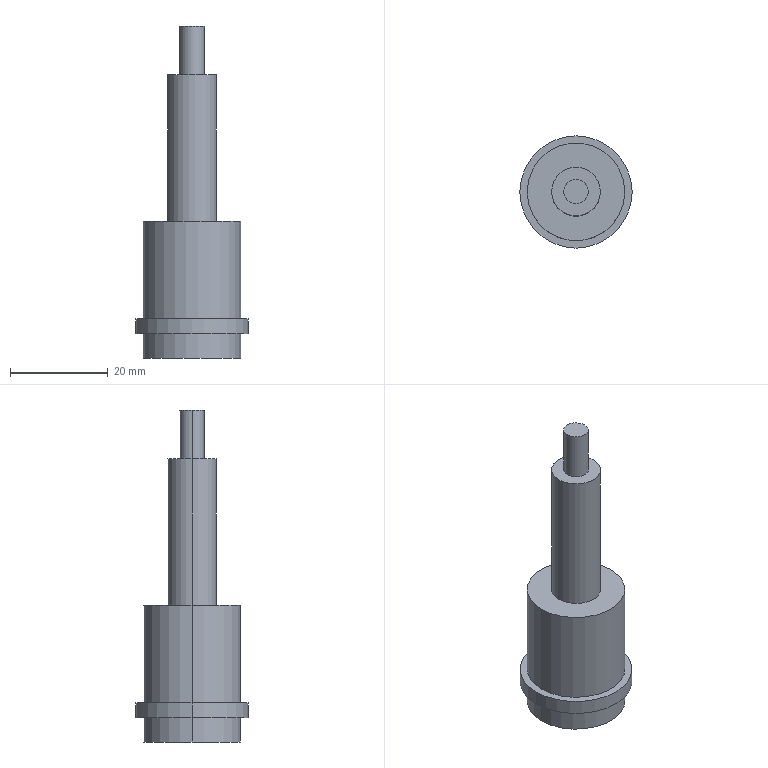Part | SolidWorks | features ICE 4, Extrusion 1 | 1 solid | 16 faces | box 23 x 23 x 68 mm | volume 11653 mm3 | cylinder 10 | plane 6 | commonest cylinder face diameters 20 x4 5 x2 10 x2 23 x2
STEP:
#1=CARTESIAN_POINT('',(2.5,0.,68.));
#2=VERTEX_POINT('',#1);
#3=CARTESIAN_POINT('',(-2.5,0.,68.));
#4=VERTEX_POINT('',#3);
#5=CARTESIAN_POINT('',(0.,0.,68.));
#6=DIRECTION('',(0.,0.,1.));
#7=DIRECTION('',(1.,0.,0.));
#8=AXIS2_PLACEMENT_3D('',#5,#6,#7);
#9=CIRCLE('',#8,2.5);
#10=EDGE_CURVE('',#2,#4,#9,.T.);
#11=ORIENTED_EDGE('',*,*,#10,.F.);
#12=CARTESIAN_POINT('',(2.5,0.,58.));
#13=VERTEX_POINT('',#12);
#14=CARTESIAN_POINT('',(2.5,0.,68.));
#15=DIRECTION('',(0.,0.,-1.));
#16=VECTOR('',#15,1000.);
#17=LINE('',#14,#16);
#18=EDGE_CURVE('',#2,#13,#17,.T.);
#19=ORIENTED_EDGE('',*,*,#18,.T.);
#20=CARTESIAN_POINT('',(-2.5,0.,58.));
#21=VERTEX_POINT('',#20);
#22=CARTESIAN_POINT('',(0.,0.,58.));
#23=DIRECTION('',(0.,0.,1.));
#24=DIRECTION('',(1.,0.,0.));
#25=AXIS2_PLACEMENT_3D('',#22,#23,#24);
#26=CIRCLE('',#25,2.5);
#27=EDGE_CURVE('',#13,#21,#26,.T.);
#28=ORIENTED_EDGE('',*,*,#27,.T.);
#29=CARTESIAN_POINT('',(-2.5,0.,68.));
#30=DIRECTION('',(0.,0.,-1.));
#31=VECTOR('',#30,1000.);
#32=LINE('',#29,#31);
#33=EDGE_CURVE('',#4,#21,#32,.T.);
#34=ORIENTED_EDGE('',*,*,#33,.F.);
#35=EDGE_LOOP('',(#11,#19,#28,#34));
#36=FACE_OUTER_BOUND('',#35,.T.);
#37=CARTESIAN_POINT('',(0.,0.,68.));
#38=DIRECTION('',(0.,0.,-1.));
#39=DIRECTION('',(-1.,0.,0.));
#40=AXIS2_PLACEMENT_3D('',#37,#38,#39);
#41=CYLINDRICAL_SURFACE('',#40,2.5);
#42=ADVANCED_FACE('',(#36),#41,.T.);
#43=CARTESIAN_POINT('',(5.,0.,58.));
#44=VERTEX_POINT('',#43);
#45=CARTESIAN_POINT('',(-5.,0.,58.));
#46=VERTEX_POINT('',#45);
#47=CARTESIAN_POINT('',(0.,0.,58.));
#48=DIRECTION('',(0.,0.,1.));
#49=DIRECTION('',(1.,0.,0.));
#50=AXIS2_PLACEMENT_3D('',#47,#48,#49);
#51=CIRCLE('',#50,5.);
#52=EDGE_CURVE('',#44,#46,#51,.T.);
#53=ORIENTED_EDGE('',*,*,#52,.F.);
#54=CARTESIAN_POINT('',(5.,0.,28.));
#55=VERTEX_POINT('',#54);
#56=CARTESIAN_POINT('',(5.,0.,58.));
#57=DIRECTION('',(0.,0.,-1.));
#58=VECTOR('',#57,1000.);
#59=LINE('',#56,#58);
#60=EDGE_CURVE('',#44,#55,#59,.T.);
#61=ORIENTED_EDGE('',*,*,#60,.T.);
#62=CARTESIAN_POINT('',(-5.,0.,28.));
#63=VERTEX_POINT('',#62);
#64=CARTESIAN_POINT('',(0.,0.,28.));
#65=DIRECTION('',(0.,0.,1.));
#66=DIRECTION('',(1.,0.,0.));
#67=AXIS2_PLACEMENT_3D('',#64,#65,#66);
#68=CIRCLE('',#67,5.);
#69=EDGE_CURVE('',#55,#63,#68,.T.);
#70=ORIENTED_EDGE('',*,*,#69,.T.);
#71=CARTESIAN_POINT('',(-5.,0.,58.));
#72=DIRECTION('',(0.,0.,-1.));
#73=VECTOR('',#72,1000.);
#74=LINE('',#71,#73);
#75=EDGE_CURVE('',#46,#63,#74,.T.);
#76=ORIENTED_EDGE('',*,*,#75,.F.);
#77=EDGE_LOOP('',(#53,#61,#70,#76));
#78=FACE_OUTER_BOUND('',#77,.T.);
#79=CARTESIAN_POINT('',(0.,0.,58.));
#80=DIRECTION('',(0.,0.,-1.));
#81=DIRECTION('',(-1.,0.,0.));
#82=AXIS2_PLACEMENT_3D('',#79,#80,#81);
#83=CYLINDRICAL_SURFACE('',#82,5.);
#84=ADVANCED_FACE('',(#78),#83,.T.);
#85=CARTESIAN_POINT('',(10.,0.,28.));
#86=VERTEX_POINT('',#85);
#87=CARTESIAN_POINT('',(-10.,0.,28.));
#88=VERTEX_POINT('',#87);
#89=CARTESIAN_POINT('',(0.,0.,28.));
#90=DIRECTION('',(0.,0.,1.));
#91=DIRECTION('',(1.,0.,0.));
#92=AXIS2_PLACEMENT_3D('',#89,#90,#91);
#93=CIRCLE('',#92,10.);
#94=EDGE_CURVE('',#86,#88,#93,.T.);
#95=ORIENTED_EDGE('',*,*,#94,.F.);
#96=CARTESIAN_POINT('',(10.,0.,8.));
#97=VERTEX_POINT('',#96);
#98=CARTESIAN_POINT('',(10.,0.,28.));
#99=DIRECTION('',(0.,0.,-1.));
#100=VECTOR('',#99,1000.);
#101=LINE('',#98,#100);
#102=EDGE_CURVE('',#86,#97,#101,.T.);
#103=ORIENTED_EDGE('',*,*,#102,.T.);
#104=CARTESIAN_POINT('',(-10.,0.,8.));
#105=VERTEX_POINT('',#104);
#106=CARTESIAN_POINT('',(0.,0.,8.));
#107=DIRECTION('',(0.,0.,1.));
#108=DIRECTION('',(1.,0.,0.));
#109=AXIS2_PLACEMENT_3D('',#106,#107,#108);
#110=CIRCLE('',#109,10.);
#111=EDGE_CURVE('',#97,#105,#110,.T.);
#112=ORIENTED_EDGE('',*,*,#111,.T.);
#113=CARTESIAN_POINT('',(-10.,0.,28.));
#114=DIRECTION('',(0.,0.,-1.));
#115=VECTOR('',#114,1000.);
#116=LINE('',#113,#115);
#117=EDGE_CURVE('',#88,#105,#116,.T.);
#118=ORIENTED_EDGE('',*,*,#117,.F.);
#119=EDGE_LOOP('',(#95,#103,#112,#118));
#120=FACE_OUTER_BOUND('',#119,.T.);
#121=CARTESIAN_POINT('',(0.,0.,28.));
#122=DIRECTION('',(0.,0.,-1.));
#123=DIRECTION('',(-1.,0.,0.));
#124=AXIS2_PLACEMENT_3D('',#121,#122,#123);
#125=CYLINDRICAL_SURFACE('',#124,10.);
#126=ADVANCED_FACE('',(#120),#125,.T.);
#127=CARTESIAN_POINT('',(11.5,0.,8.));
#128=VERTEX_POINT('',#127);
#129=CARTESIAN_POINT('',(-11.5,0.,8.));
#130=VERTEX_POINT('',#129);
#131=CARTESIAN_POINT('',(0.,0.,8.));
#132=DIRECTION('',(0.,0.,1.));
#133=DIRECTION('',(1.,0.,0.));
#134=AXIS2_PLACEMENT_3D('',#131,#132,#133);
#135=CIRCLE('',#134,11.5);
#136=EDGE_CURVE('',#128,#130,#135,.T.);
#137=ORIENTED_EDGE('',*,*,#136,.F.);
#138=CARTESIAN_POINT('',(11.5,0.,5.));
#139=VERTEX_POINT('',#138);
#140=CARTESIAN_POINT('',(11.5,0.,8.));
#141=DIRECTION('',(0.,0.,-1.));
#142=VECTOR('',#141,1000.);
#143=LINE('',#140,#142);
#144=EDGE_CURVE('',#128,#139,#143,.T.);
#145=ORIENTED_EDGE('',*,*,#144,.T.);
#146=CARTESIAN_POINT('',(-11.5,0.,5.));
#147=VERTEX_POINT('',#146);
#148=CARTESIAN_POINT('',(0.,0.,5.));
#149=DIRECTION('',(0.,0.,1.));
#150=DIRECTION('',(1.,0.,0.));
#151=AXIS2_PLACEMENT_3D('',#148,#149,#150);
#152=CIRCLE('',#151,11.5);
#153=EDGE_CURVE('',#139,#147,#152,.T.);
#154=ORIENTED_EDGE('',*,*,#153,.T.);
#155=CARTESIAN_POINT('',(-11.5,0.,8.));
#156=DIRECTION('',(0.,0.,-1.));
#157=VECTOR('',#156,1000.);
#158=LINE('',#155,#157);
#159=EDGE_CURVE('',#130,#147,#158,.T.);
#160=ORIENTED_EDGE('',*,*,#159,.F.);
#161=EDGE_LOOP('',(#137,#145,#154,#160));
#162=FACE_OUTER_BOUND('',#161,.T.);
#163=CARTESIAN_POINT('',(0.,0.,8.));
#164=DIRECTION('',(0.,0.,-1.));
#165=DIRECTION('',(-1.,0.,0.));
#166=AXIS2_PLACEMENT_3D('',#163,#164,#165);
#167=CYLINDRICAL_SURFACE('',#166,11.5);
#168=ADVANCED_FACE('',(#162),#167,.T.);
#169=CARTESIAN_POINT('',(10.,0.,5.));
#170=VERTEX_POINT('',#169);
#171=CARTESIAN_POINT('',(-10.,0.,5.));
#172=VERTEX_POINT('',#171);
#173=CARTESIAN_POINT('',(0.,0.,5.));
#174=DIRECTION('',(0.,0.,1.));
#175=DIRECTION('',(1.,0.,0.));
#176=AXIS2_PLACEMENT_3D('',#173,#174,#175);
#177=CIRCLE('',#176,10.);
#178=EDGE_CURVE('',#170,#172,#177,.T.);
#179=ORIENTED_EDGE('',*,*,#178,.F.);
#180=CARTESIAN_POINT('',(10.,0.,0.));
#181=VERTEX_POINT('',#180);
#182=CARTESIAN_POINT('',(10.,0.,5.));
#183=DIRECTION('',(0.,0.,-1.));
#184=VECTOR('',#183,1000.);
#185=LINE('',#182,#184);
#186=EDGE_CURVE('',#170,#181,#185,.T.);
#187=ORIENTED_EDGE('',*,*,#186,.T.);
#188=CARTESIAN_POINT('',(-10.,0.,0.));
#189=VERTEX_POINT('',#188);
#190=CARTESIAN_POINT('',(0.,0.,0.));
#191=DIRECTION('',(0.,0.,1.));
#192=DIRECTION('',(1.,0.,0.));
#193=AXIS2_PLACEMENT_3D('',#190,#191,#192);
#194=CIRCLE('',#193,10.);
#195=EDGE_CURVE('',#181,#189,#194,.T.);
#196=ORIENTED_EDGE('',*,*,#195,.T.);
#197=CARTESIAN_POINT('',(-10.,0.,5.));
#198=DIRECTION('',(0.,0.,-1.));
#199=VECTOR('',#198,1000.);
#200=LINE('',#197,#199);
#201=EDGE_CURVE('',#172,#189,#200,.T.);
#202=ORIENTED_EDGE('',*,*,#201,.F.);
#203=EDGE_LOOP('',(#179,#187,#196,#202));
#204=FACE_OUTER_BOUND('',#203,.T.);
#205=CARTESIAN_POINT('',(0.,0.,5.));
#206=DIRECTION('',(0.,0.,-1.));
#207=DIRECTION('',(-1.,0.,0.));
#208=AXIS2_PLACEMENT_3D('',#205,#206,#207);
#209=CYLINDRICAL_SURFACE('',#208,10.);
#210=ADVANCED_FACE('',(#204),#209,.T.);
#211=ORIENTED_EDGE('',*,*,#186,.F.);
#212=CARTESIAN_POINT('',(0.,0.,5.));
#213=DIRECTION('',(0.,0.,1.));
#214=DIRECTION('',(1.,0.,0.));
#215=AXIS2_PLACEMENT_3D('',#212,#213,#214);
#216=CIRCLE('',#215,10.);
#217=EDGE_CURVE('',#172,#170,#216,.T.);
#218=ORIENTED_EDGE('',*,*,#217,.F.);
#219=ORIENTED_EDGE('',*,*,#201,.T.);
#220=CARTESIAN_POINT('',(0.,0.,0.));
#221=DIRECTION('',(0.,0.,1.));
#222=DIRECTION('',(1.,0.,0.));
#223=AXIS2_PLACEMENT_3D('',#220,#221,#222);
#224=CIRCLE('',#223,10.);
#225=EDGE_CURVE('',#189,#181,#224,.T.);
#226=ORIENTED_EDGE('',*,*,#225,.T.);
#227=EDGE_LOOP('',(#211,#218,#219,#226));
#228=FACE_OUTER_BOUND('',#227,.T.);
#229=CARTESIAN_POINT('',(0.,0.,5.));
#230=DIRECTION('',(0.,0.,-1.));
#231=DIRECTION('',(-1.,0.,0.));
#232=AXIS2_PLACEMENT_3D('',#229,#230,#231);
#233=CYLINDRICAL_SURFACE('',#232,10.);
#234=ADVANCED_FACE('',(#228),#233,.T.);
#235=ORIENTED_EDGE('',*,*,#225,.F.);
#236=ORIENTED_EDGE('',*,*,#195,.F.);
#237=EDGE_LOOP('',(#235,#236));
#238=FACE_OUTER_BOUND('',#237,.T.);
#239=CARTESIAN_POINT('',(0.,0.,0.));
#240=DIRECTION('',(0.,0.,1.));
#241=DIRECTION('',(1.,0.,0.));
#242=AXIS2_PLACEMENT_3D('',#239,#240,#241);
#243=PLANE('',#242);
#244=ADVANCED_FACE('',(#238),#243,.F.);
#245=ORIENTED_EDGE('',*,*,#144,.F.);
#246=CARTESIAN_POINT('',(0.,0.,8.));
#247=DIRECTION('',(0.,0.,1.));
#248=DIRECTION('',(1.,0.,0.));
#249=AXIS2_PLACEMENT_3D('',#246,#247,#248);
#250=CIRCLE('',#249,11.5);
#251=EDGE_CURVE('',#130,#128,#250,.T.);
#252=ORIENTED_EDGE('',*,*,#251,.F.);
#253=ORIENTED_EDGE('',*,*,#159,.T.);
#254=CARTESIAN_POINT('',(0.,0.,5.));
#255=DIRECTION('',(0.,0.,1.));
#256=DIRECTION('',(1.,0.,0.));
#257=AXIS2_PLACEMENT_3D('',#254,#255,#256);
#258=CIRCLE('',#257,11.5);
#259=EDGE_CURVE('',#147,#139,#258,.T.);
#260=ORIENTED_EDGE('',*,*,#259,.T.);
#261=EDGE_LOOP('',(#245,#252,#253,#260));
#262=FACE_OUTER_BOUND('',#261,.T.);
#263=CARTESIAN_POINT('',(0.,0.,8.));
#264=DIRECTION('',(0.,0.,-1.));
#265=DIRECTION('',(-1.,0.,0.));
#266=AXIS2_PLACEMENT_3D('',#263,#264,#265);
#267=CYLINDRICAL_SURFACE('',#266,11.5);
#268=ADVANCED_FACE('',(#262),#267,.T.);
#269=CARTESIAN_POINT('',(0.,0.,8.));
#270=DIRECTION('',(0.,0.,1.));
#271=DIRECTION('',(1.,0.,0.));
#272=AXIS2_PLACEMENT_3D('',#269,#270,#271);
#273=CIRCLE('',#272,10.);
#274=EDGE_CURVE('',#105,#97,#273,.T.);
#275=ORIENTED_EDGE('',*,*,#274,.F.);
#276=ORIENTED_EDGE('',*,*,#111,.F.);
#277=EDGE_LOOP('',(#275,#276));
#278=FACE_BOUND('',#277,.T.);
#279=ORIENTED_EDGE('',*,*,#251,.T.);
#280=ORIENTED_EDGE('',*,*,#136,.T.);
#281=EDGE_LOOP('',(#279,#280));
#282=FACE_OUTER_BOUND('',#281,.T.);
#283=CARTESIAN_POINT('',(0.,0.,8.));
#284=DIRECTION('',(0.,0.,1.));
#285=DIRECTION('',(1.,0.,0.));
#286=AXIS2_PLACEMENT_3D('',#283,#284,#285);
#287=PLANE('',#286);
#288=ADVANCED_FACE('',(#278,#282),#287,.T.);
#289=ORIENTED_EDGE('',*,*,#217,.T.);
#290=ORIENTED_EDGE('',*,*,#178,.T.);
#291=EDGE_LOOP('',(#289,#290));
#292=FACE_BOUND('',#291,.T.);
#293=ORIENTED_EDGE('',*,*,#259,.F.);
#294=ORIENTED_EDGE('',*,*,#153,.F.);
#295=EDGE_LOOP('',(#293,#294));
#296=FACE_OUTER_BOUND('',#295,.T.);
#297=CARTESIAN_POINT('',(0.,0.,5.));
#298=DIRECTION('',(0.,0.,1.));
#299=DIRECTION('',(1.,0.,0.));
#300=AXIS2_PLACEMENT_3D('',#297,#298,#299);
#301=PLANE('',#300);
#302=ADVANCED_FACE('',(#292,#296),#301,.F.);
#303=ORIENTED_EDGE('',*,*,#102,.F.);
#304=CARTESIAN_POINT('',(0.,0.,28.));
#305=DIRECTION('',(0.,0.,1.));
#306=DIRECTION('',(1.,0.,0.));
#307=AXIS2_PLACEMENT_3D('',#304,#305,#306);
#308=CIRCLE('',#307,10.);
#309=EDGE_CURVE('',#88,#86,#308,.T.);
#310=ORIENTED_EDGE('',*,*,#309,.F.);
#311=ORIENTED_EDGE('',*,*,#117,.T.);
#312=ORIENTED_EDGE('',*,*,#274,.T.);
#313=EDGE_LOOP('',(#303,#310,#311,#312));
#314=FACE_OUTER_BOUND('',#313,.T.);
#315=CARTESIAN_POINT('',(0.,0.,28.));
#316=DIRECTION('',(0.,0.,-1.));
#317=DIRECTION('',(-1.,0.,0.));
#318=AXIS2_PLACEMENT_3D('',#315,#316,#317);
#319=CYLINDRICAL_SURFACE('',#318,10.);
#320=ADVANCED_FACE('',(#314),#319,.T.);
#321=CARTESIAN_POINT('',(0.,0.,28.));
#322=DIRECTION('',(0.,0.,1.));
#323=DIRECTION('',(1.,0.,0.));
#324=AXIS2_PLACEMENT_3D('',#321,#322,#323);
#325=CIRCLE('',#324,5.);
#326=EDGE_CURVE('',#63,#55,#325,.T.);
#327=ORIENTED_EDGE('',*,*,#326,.F.);
#328=ORIENTED_EDGE('',*,*,#69,.F.);
#329=EDGE_LOOP('',(#327,#328));
#330=FACE_BOUND('',#329,.T.);
#331=ORIENTED_EDGE('',*,*,#309,.T.);
#332=ORIENTED_EDGE('',*,*,#94,.T.);
#333=EDGE_LOOP('',(#331,#332));
#334=FACE_OUTER_BOUND('',#333,.T.);
#335=CARTESIAN_POINT('',(0.,0.,28.));
#336=DIRECTION('',(0.,0.,1.));
#337=DIRECTION('',(1.,0.,0.));
#338=AXIS2_PLACEMENT_3D('',#335,#336,#337);
#339=PLANE('',#338);
#340=ADVANCED_FACE('',(#330,#334),#339,.T.);
#341=ORIENTED_EDGE('',*,*,#60,.F.);
#342=CARTESIAN_POINT('',(0.,0.,58.));
#343=DIRECTION('',(0.,0.,1.));
#344=DIRECTION('',(1.,0.,0.));
#345=AXIS2_PLACEMENT_3D('',#342,#343,#344);
#346=CIRCLE('',#345,5.);
#347=EDGE_CURVE('',#46,#44,#346,.T.);
#348=ORIENTED_EDGE('',*,*,#347,.F.);
#349=ORIENTED_EDGE('',*,*,#75,.T.);
#350=ORIENTED_EDGE('',*,*,#326,.T.);
#351=EDGE_LOOP('',(#341,#348,#349,#350));
#352=FACE_OUTER_BOUND('',#351,.T.);
#353=CARTESIAN_POINT('',(0.,0.,58.));
#354=DIRECTION('',(0.,0.,-1.));
#355=DIRECTION('',(-1.,0.,0.));
#356=AXIS2_PLACEMENT_3D('',#353,#354,#355);
#357=CYLINDRICAL_SURFACE('',#356,5.);
#358=ADVANCED_FACE('',(#352),#357,.T.);
#359=CARTESIAN_POINT('',(0.,0.,58.));
#360=DIRECTION('',(0.,0.,1.));
#361=DIRECTION('',(1.,0.,0.));
#362=AXIS2_PLACEMENT_3D('',#359,#360,#361);
#363=CIRCLE('',#362,2.5);
#364=EDGE_CURVE('',#21,#13,#363,.T.);
#365=ORIENTED_EDGE('',*,*,#364,.F.);
#366=ORIENTED_EDGE('',*,*,#27,.F.);
#367=EDGE_LOOP('',(#365,#366));
#368=FACE_BOUND('',#367,.T.);
#369=ORIENTED_EDGE('',*,*,#347,.T.);
#370=ORIENTED_EDGE('',*,*,#52,.T.);
#371=EDGE_LOOP('',(#369,#370));
#372=FACE_OUTER_BOUND('',#371,.T.);
#373=CARTESIAN_POINT('',(0.,0.,58.));
#374=DIRECTION('',(0.,0.,1.));
#375=DIRECTION('',(1.,0.,0.));
#376=AXIS2_PLACEMENT_3D('',#373,#374,#375);
#377=PLANE('',#376);
#378=ADVANCED_FACE('',(#368,#372),#377,.T.);
#379=ORIENTED_EDGE('',*,*,#18,.F.);
#380=CARTESIAN_POINT('',(0.,0.,68.));
#381=DIRECTION('',(0.,0.,1.));
#382=DIRECTION('',(1.,0.,0.));
#383=AXIS2_PLACEMENT_3D('',#380,#381,#382);
#384=CIRCLE('',#383,2.5);
#385=EDGE_CURVE('',#4,#2,#384,.T.);
#386=ORIENTED_EDGE('',*,*,#385,.F.);
#387=ORIENTED_EDGE('',*,*,#33,.T.);
#388=ORIENTED_EDGE('',*,*,#364,.T.);
#389=EDGE_LOOP('',(#379,#386,#387,#388));
#390=FACE_OUTER_BOUND('',#389,.T.);
#391=CARTESIAN_POINT('',(0.,0.,68.));
#392=DIRECTION('',(0.,0.,-1.));
#393=DIRECTION('',(-1.,0.,0.));
#394=AXIS2_PLACEMENT_3D('',#391,#392,#393);
#395=CYLINDRICAL_SURFACE('',#394,2.5);
#396=ADVANCED_FACE('',(#390),#395,.T.);
#397=ORIENTED_EDGE('',*,*,#385,.T.);
#398=ORIENTED_EDGE('',*,*,#10,.T.);
#399=EDGE_LOOP('',(#397,#398));
#400=FACE_OUTER_BOUND('',#399,.T.);
#401=CARTESIAN_POINT('',(0.,0.,68.));
#402=DIRECTION('',(0.,0.,1.));
#403=DIRECTION('',(1.,0.,0.));
#404=AXIS2_PLACEMENT_3D('',#401,#402,#403);
#405=PLANE('',#404);
#406=ADVANCED_FACE('',(#400),#405,.T.);
#407=CLOSED_SHELL('',(#42,#84,#126,#168,#210,#234,#244,#268,#288,#302,#320,#340,#358,#378,#396,#406));
#408=MANIFOLD_SOLID_BREP('',#407);
#409=CARTESIAN_POINT('',(0.,0.,0.));
#410=DIRECTION('',(0.,0.,1.));
#411=DIRECTION('',(1.,0.,0.));
#412=AXIS2_PLACEMENT_3D('',#409,#410,#411);
#413=(LENGTH_UNIT()NAMED_UNIT(*)SI_UNIT(.MILLI.,.METRE.));
#414=UNCERTAINTY_MEASURE_WITH_UNIT(LENGTH_MEASURE(0.00001),#413,'','');
#415=(NAMED_UNIT(*)PLANE_ANGLE_UNIT()SI_UNIT($,.RADIAN.));
#416=(NAMED_UNIT(*)SI_UNIT($,.STERADIAN.)SOLID_ANGLE_UNIT());
#417=(GEOMETRIC_REPRESENTATION_CONTEXT(3)GLOBAL_UNCERTAINTY_ASSIGNED_CONTEXT((#414))GLOBAL_UNIT_ASSIGNED_CONTEXT((#413,#415,#416))REPRESENTATION_CONTEXT('',''));
#418=ADVANCED_BREP_SHAPE_REPRESENTATION('',(#408,#412),#417);